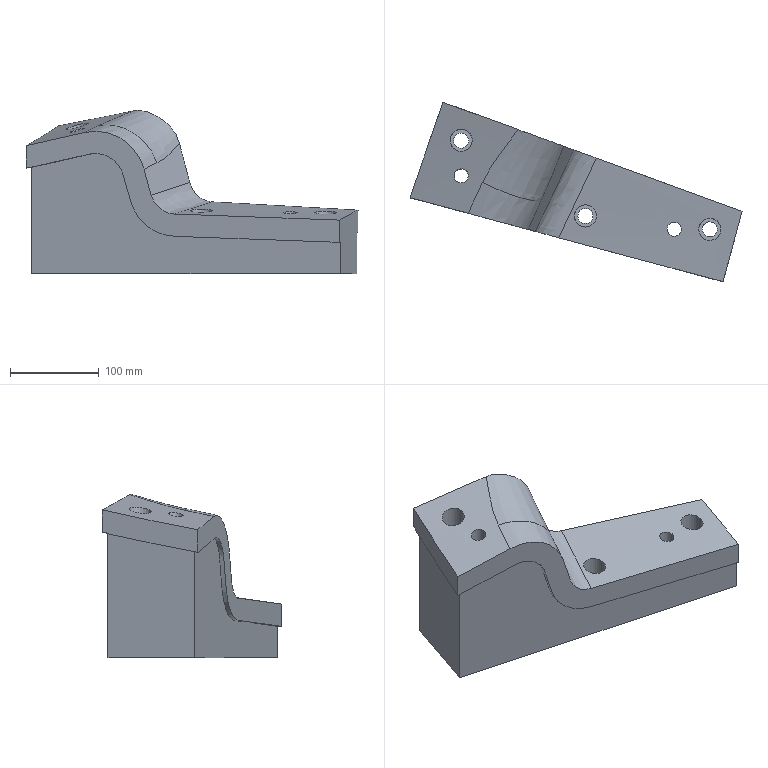Part | NX | features solid 2 | 1 solid | 28 faces | box 373.871 x 202.071 x 183.776 mm | volume 3420058 mm3 | plane 11 | spline 9 | cylinder 8 | commonest cylinder face diameters 17 x3 25 x3 16 x2